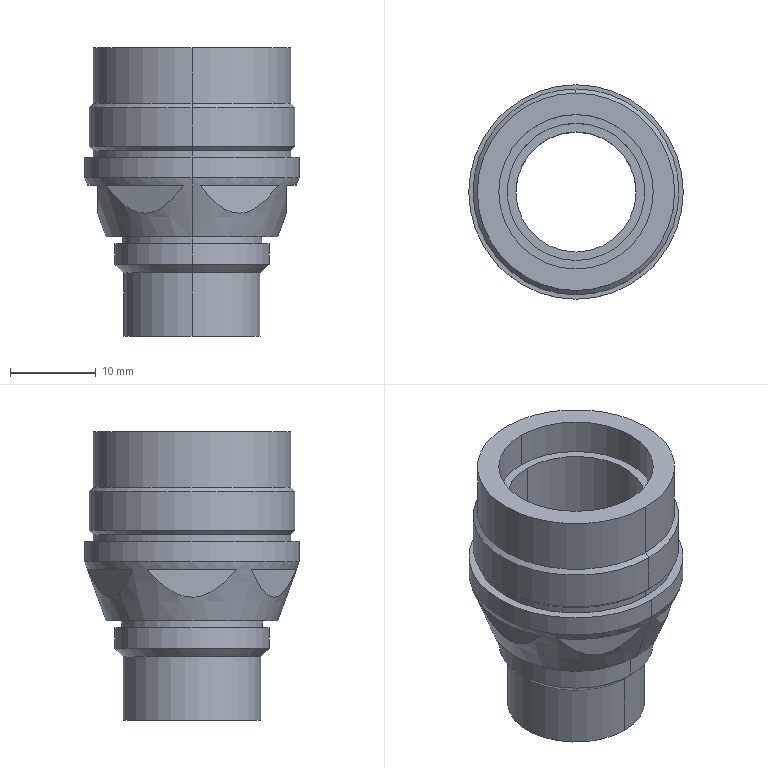Part | STEP file | ASND-0110-4216109900 | 1 solid | 47 faces | box 25 x 25 x 33.65 mm | volume 5833 mm3 | cylinder 20 | plane 19 | cone 8 | commonest cylinder face diameters 16 x4 18 x4 23 x4 14 x2 16.4 x2 24 x2